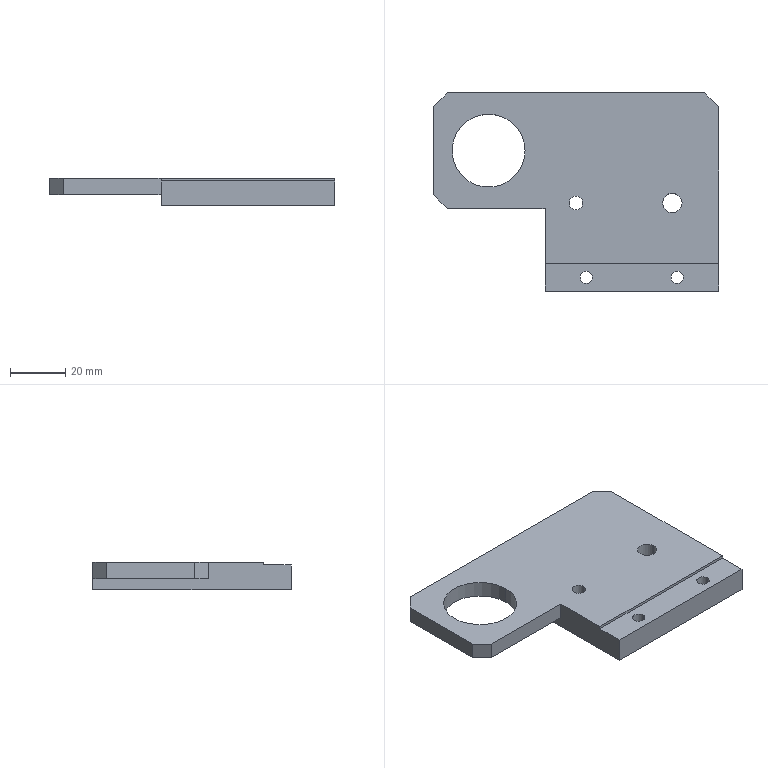Part | STEP file | 2035 Cylinder mounting seat 1 | 1 solid | 30 faces | box 103.5 x 72 x 10 mm | volume 50168 mm3 | plane 16 | cylinder 14 | commonest cylinder face diameters 4.5 x4 8 x4 5 x2 7 x2 26.5 x2